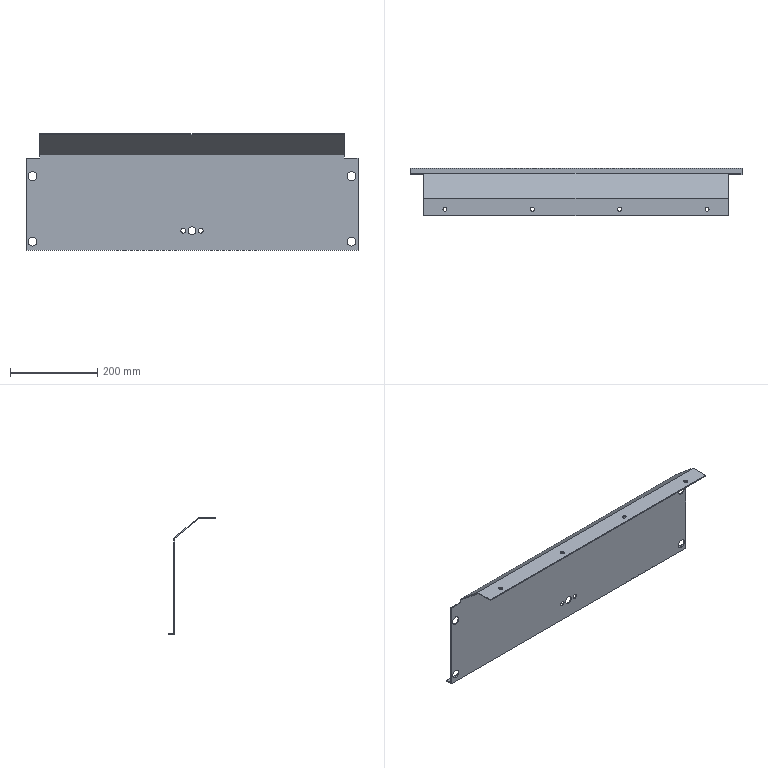Part | SolidWorks | features BaseBody 1 | 1 solid | 38 faces | box 760 x 109.5 x 267.5 mm | volume 630879 mm3 | cylinder 22 | plane 16 | commonest cylinder face diameters 9.1 x8 20 x8 11 x4 18 x2
STEP:
#1=CARTESIAN_POINT('',(181.946,-3035.973,2024.971));
#2=VERTEX_POINT('',#1);
#3=CARTESIAN_POINT('',(181.946,-3035.973,2004.971));
#4=VERTEX_POINT('',#3);
#5=CARTESIAN_POINT('',(181.946,-3035.973,2014.971));
#6=DIRECTION('',(0.,-1.,0.));
#7=DIRECTION('',(0.,0.,-1.));
#8=AXIS2_PLACEMENT_3D('',#5,#6,#7);
#9=CIRCLE('',#8,10.);
#10=EDGE_CURVE('',#2,#4,#9,.T.);
#11=ORIENTED_EDGE('',*,*,#10,.F.);
#12=CARTESIAN_POINT('',(181.946,-3038.473,2024.971));
#13=VERTEX_POINT('',#12);
#14=CARTESIAN_POINT('',(181.946,-3041.02,2024.971));
#15=DIRECTION('',(0.,-1.,0.));
#16=VECTOR('',#15,1000.);
#17=LINE('',#14,#16);
#18=EDGE_CURVE('',#2,#13,#17,.T.);
#19=ORIENTED_EDGE('',*,*,#18,.T.);
#20=CARTESIAN_POINT('',(181.946,-3038.473,2004.971));
#21=VERTEX_POINT('',#20);
#22=CARTESIAN_POINT('',(181.946,-3038.473,2014.971));
#23=DIRECTION('',(0.,1.,0.));
#24=DIRECTION('',(0.,0.,-1.));
#25=AXIS2_PLACEMENT_3D('',#22,#23,#24);
#26=CIRCLE('',#25,10.);
#27=EDGE_CURVE('',#21,#13,#26,.T.);
#28=ORIENTED_EDGE('',*,*,#27,.F.);
#29=CARTESIAN_POINT('',(181.946,-3041.02,2004.971));
#30=DIRECTION('',(0.,-1.,0.));
#31=VECTOR('',#30,1000.);
#32=LINE('',#29,#31);
#33=EDGE_CURVE('',#4,#21,#32,.T.);
#34=ORIENTED_EDGE('',*,*,#33,.F.);
#35=EDGE_LOOP('',(#11,#19,#28,#34));
#36=FACE_OUTER_BOUND('',#35,.T.);
#37=CARTESIAN_POINT('',(181.946,-3041.02,2014.971));
#38=DIRECTION('',(0.,-1.,0.));
#39=DIRECTION('',(0.,0.,-1.));
#40=AXIS2_PLACEMENT_3D('',#37,#38,#39);
#41=CYLINDRICAL_SURFACE('',#40,10.);
#42=ADVANCED_FACE('',(#36),#41,.F.);
#43=CARTESIAN_POINT('',(911.946,-3038.473,2004.971));
#44=VERTEX_POINT('',#43);
#45=CARTESIAN_POINT('',(911.946,-3038.473,2024.971));
#46=VERTEX_POINT('',#45);
#47=CARTESIAN_POINT('',(911.946,-3038.473,2014.971));
#48=DIRECTION('',(0.,1.,0.));
#49=DIRECTION('',(0.,0.,1.));
#50=AXIS2_PLACEMENT_3D('',#47,#48,#49);
#51=CIRCLE('',#50,10.);
#52=EDGE_CURVE('',#44,#46,#51,.T.);
#53=ORIENTED_EDGE('',*,*,#52,.F.);
#54=CARTESIAN_POINT('',(911.946,-3035.973,2004.971));
#55=VERTEX_POINT('',#54);
#56=CARTESIAN_POINT('',(911.946,-3041.02,2004.971));
#57=DIRECTION('',(0.,1.,0.));
#58=VECTOR('',#57,1000.);
#59=LINE('',#56,#58);
#60=EDGE_CURVE('',#44,#55,#59,.T.);
#61=ORIENTED_EDGE('',*,*,#60,.T.);
#62=CARTESIAN_POINT('',(911.946,-3035.973,2024.971));
#63=VERTEX_POINT('',#62);
#64=CARTESIAN_POINT('',(911.946,-3035.973,2014.971));
#65=DIRECTION('',(0.,-1.,0.));
#66=DIRECTION('',(0.,0.,1.));
#67=AXIS2_PLACEMENT_3D('',#64,#65,#66);
#68=CIRCLE('',#67,10.);
#69=EDGE_CURVE('',#63,#55,#68,.T.);
#70=ORIENTED_EDGE('',*,*,#69,.F.);
#71=CARTESIAN_POINT('',(911.946,-3041.02,2024.971));
#72=DIRECTION('',(0.,1.,0.));
#73=VECTOR('',#72,1000.);
#74=LINE('',#71,#73);
#75=EDGE_CURVE('',#46,#63,#74,.T.);
#76=ORIENTED_EDGE('',*,*,#75,.F.);
#77=EDGE_LOOP('',(#53,#61,#70,#76));
#78=FACE_OUTER_BOUND('',#77,.T.);
#79=CARTESIAN_POINT('',(911.946,-3041.02,2014.971));
#80=DIRECTION('',(0.,1.,0.));
#81=DIRECTION('',(0.,0.,1.));
#82=AXIS2_PLACEMENT_3D('',#79,#80,#81);
#83=CYLINDRICAL_SURFACE('',#82,10.);
#84=ADVANCED_FACE('',(#78),#83,.F.);
#85=CARTESIAN_POINT('',(911.946,-3038.473,1854.971));
#86=VERTEX_POINT('',#85);
#87=CARTESIAN_POINT('',(911.946,-3038.473,1874.971));
#88=VERTEX_POINT('',#87);
#89=CARTESIAN_POINT('',(911.946,-3038.473,1864.971));
#90=DIRECTION('',(0.,1.,0.));
#91=DIRECTION('',(0.,0.,1.));
#92=AXIS2_PLACEMENT_3D('',#89,#90,#91);
#93=CIRCLE('',#92,10.);
#94=EDGE_CURVE('',#86,#88,#93,.T.);
#95=ORIENTED_EDGE('',*,*,#94,.F.);
#96=CARTESIAN_POINT('',(911.946,-3035.973,1854.971));
#97=VERTEX_POINT('',#96);
#98=CARTESIAN_POINT('',(911.946,-3041.02,1854.971));
#99=DIRECTION('',(0.,1.,0.));
#100=VECTOR('',#99,1000.);
#101=LINE('',#98,#100);
#102=EDGE_CURVE('',#86,#97,#101,.T.);
#103=ORIENTED_EDGE('',*,*,#102,.T.);
#104=CARTESIAN_POINT('',(911.946,-3035.973,1874.971));
#105=VERTEX_POINT('',#104);
#106=CARTESIAN_POINT('',(911.946,-3035.973,1864.971));
#107=DIRECTION('',(0.,-1.,0.));
#108=DIRECTION('',(0.,0.,1.));
#109=AXIS2_PLACEMENT_3D('',#106,#107,#108);
#110=CIRCLE('',#109,10.);
#111=EDGE_CURVE('',#105,#97,#110,.T.);
#112=ORIENTED_EDGE('',*,*,#111,.F.);
#113=CARTESIAN_POINT('',(911.946,-3041.02,1874.971));
#114=DIRECTION('',(0.,1.,0.));
#115=VECTOR('',#114,1000.);
#116=LINE('',#113,#115);
#117=EDGE_CURVE('',#88,#105,#116,.T.);
#118=ORIENTED_EDGE('',*,*,#117,.F.);
#119=EDGE_LOOP('',(#95,#103,#112,#118));
#120=FACE_OUTER_BOUND('',#119,.T.);
#121=CARTESIAN_POINT('',(911.946,-3041.02,1864.971));
#122=DIRECTION('',(0.,1.,0.));
#123=DIRECTION('',(0.,0.,1.));
#124=AXIS2_PLACEMENT_3D('',#121,#122,#123);
#125=CYLINDRICAL_SURFACE('',#124,10.);
#126=ADVANCED_FACE('',(#120),#125,.F.);
#127=CARTESIAN_POINT('',(181.946,-3035.973,1874.971));
#128=VERTEX_POINT('',#127);
#129=CARTESIAN_POINT('',(181.946,-3035.973,1854.971));
#130=VERTEX_POINT('',#129);
#131=CARTESIAN_POINT('',(181.946,-3035.973,1864.971));
#132=DIRECTION('',(0.,-1.,0.));
#133=DIRECTION('',(0.,0.,-1.));
#134=AXIS2_PLACEMENT_3D('',#131,#132,#133);
#135=CIRCLE('',#134,10.);
#136=EDGE_CURVE('',#128,#130,#135,.T.);
#137=ORIENTED_EDGE('',*,*,#136,.F.);
#138=CARTESIAN_POINT('',(181.946,-3038.473,1874.971));
#139=VERTEX_POINT('',#138);
#140=CARTESIAN_POINT('',(181.946,-3041.02,1874.971));
#141=DIRECTION('',(0.,-1.,0.));
#142=VECTOR('',#141,1000.);
#143=LINE('',#140,#142);
#144=EDGE_CURVE('',#128,#139,#143,.T.);
#145=ORIENTED_EDGE('',*,*,#144,.T.);
#146=CARTESIAN_POINT('',(181.946,-3038.473,1854.971));
#147=VERTEX_POINT('',#146);
#148=CARTESIAN_POINT('',(181.946,-3038.473,1864.971));
#149=DIRECTION('',(0.,1.,0.));
#150=DIRECTION('',(0.,0.,-1.));
#151=AXIS2_PLACEMENT_3D('',#148,#149,#150);
#152=CIRCLE('',#151,10.);
#153=EDGE_CURVE('',#147,#139,#152,.T.);
#154=ORIENTED_EDGE('',*,*,#153,.F.);
#155=CARTESIAN_POINT('',(181.946,-3041.02,1854.971));
#156=DIRECTION('',(0.,-1.,0.));
#157=VECTOR('',#156,1000.);
#158=LINE('',#155,#157);
#159=EDGE_CURVE('',#130,#147,#158,.T.);
#160=ORIENTED_EDGE('',*,*,#159,.F.);
#161=EDGE_LOOP('',(#137,#145,#154,#160));
#162=FACE_OUTER_BOUND('',#161,.T.);
#163=CARTESIAN_POINT('',(181.946,-3041.02,1864.971));
#164=DIRECTION('',(0.,-1.,0.));
#165=DIRECTION('',(0.,0.,-1.));
#166=AXIS2_PLACEMENT_3D('',#163,#164,#165);
#167=CYLINDRICAL_SURFACE('',#166,10.);
#168=ADVANCED_FACE('',(#162),#167,.F.);
#169=CARTESIAN_POINT('',(526.946,-3035.973,1895.471));
#170=VERTEX_POINT('',#169);
#171=CARTESIAN_POINT('',(526.946,-3035.973,1884.471));
#172=VERTEX_POINT('',#171);
#173=CARTESIAN_POINT('',(526.946,-3035.973,1889.971));
#174=DIRECTION('',(0.,-1.,0.));
#175=DIRECTION('',(0.,0.,-1.));
#176=AXIS2_PLACEMENT_3D('',#173,#174,#175);
#177=CIRCLE('',#176,5.5);
#178=EDGE_CURVE('',#170,#172,#177,.T.);
#179=ORIENTED_EDGE('',*,*,#178,.F.);
#180=CARTESIAN_POINT('',(526.946,-3038.473,1895.471));
#181=VERTEX_POINT('',#180);
#182=CARTESIAN_POINT('',(526.946,-3062.639,1895.471));
#183=DIRECTION('',(0.,-1.,0.));
#184=VECTOR('',#183,1000.);
#185=LINE('',#182,#184);
#186=EDGE_CURVE('',#170,#181,#185,.T.);
#187=ORIENTED_EDGE('',*,*,#186,.T.);
#188=CARTESIAN_POINT('',(526.946,-3038.473,1884.471));
#189=VERTEX_POINT('',#188);
#190=CARTESIAN_POINT('',(526.946,-3038.473,1889.971));
#191=DIRECTION('',(0.,1.,0.));
#192=DIRECTION('',(0.,0.,-1.));
#193=AXIS2_PLACEMENT_3D('',#190,#191,#192);
#194=CIRCLE('',#193,5.5);
#195=EDGE_CURVE('',#189,#181,#194,.T.);
#196=ORIENTED_EDGE('',*,*,#195,.F.);
#197=CARTESIAN_POINT('',(526.946,-3062.639,1884.471));
#198=DIRECTION('',(0.,-1.,0.));
#199=VECTOR('',#198,1000.);
#200=LINE('',#197,#199);
#201=EDGE_CURVE('',#172,#189,#200,.T.);
#202=ORIENTED_EDGE('',*,*,#201,.F.);
#203=EDGE_LOOP('',(#179,#187,#196,#202));
#204=FACE_OUTER_BOUND('',#203,.T.);
#205=CARTESIAN_POINT('',(526.946,-3062.639,1889.971));
#206=DIRECTION('',(0.,-1.,0.));
#207=DIRECTION('',(0.,0.,-1.));
#208=AXIS2_PLACEMENT_3D('',#205,#206,#207);
#209=CYLINDRICAL_SURFACE('',#208,5.5);
#210=ADVANCED_FACE('',(#204),#209,.F.);
#211=CARTESIAN_POINT('',(566.946,-3038.473,1884.471));
#212=VERTEX_POINT('',#211);
#213=CARTESIAN_POINT('',(566.946,-3038.473,1895.471));
#214=VERTEX_POINT('',#213);
#215=CARTESIAN_POINT('',(566.946,-3038.473,1889.971));
#216=DIRECTION('',(0.,1.,0.));
#217=DIRECTION('',(0.,0.,1.));
#218=AXIS2_PLACEMENT_3D('',#215,#216,#217);
#219=CIRCLE('',#218,5.5);
#220=EDGE_CURVE('',#212,#214,#219,.T.);
#221=ORIENTED_EDGE('',*,*,#220,.F.);
#222=CARTESIAN_POINT('',(566.946,-3035.973,1884.471));
#223=VERTEX_POINT('',#222);
#224=CARTESIAN_POINT('',(566.946,-3062.639,1884.471));
#225=DIRECTION('',(0.,1.,0.));
#226=VECTOR('',#225,1000.);
#227=LINE('',#224,#226);
#228=EDGE_CURVE('',#212,#223,#227,.T.);
#229=ORIENTED_EDGE('',*,*,#228,.T.);
#230=CARTESIAN_POINT('',(566.946,-3035.973,1895.471));
#231=VERTEX_POINT('',#230);
#232=CARTESIAN_POINT('',(566.946,-3035.973,1889.971));
#233=DIRECTION('',(0.,-1.,0.));
#234=DIRECTION('',(0.,0.,1.));
#235=AXIS2_PLACEMENT_3D('',#232,#233,#234);
#236=CIRCLE('',#235,5.5);
#237=EDGE_CURVE('',#231,#223,#236,.T.);
#238=ORIENTED_EDGE('',*,*,#237,.F.);
#239=CARTESIAN_POINT('',(566.946,-3062.639,1895.471));
#240=DIRECTION('',(0.,1.,0.));
#241=VECTOR('',#240,1000.);
#242=LINE('',#239,#241);
#243=EDGE_CURVE('',#214,#231,#242,.T.);
#244=ORIENTED_EDGE('',*,*,#243,.F.);
#245=EDGE_LOOP('',(#221,#229,#238,#244));
#246=FACE_OUTER_BOUND('',#245,.T.);
#247=CARTESIAN_POINT('',(566.946,-3062.639,1889.971));
#248=DIRECTION('',(0.,1.,0.));
#249=DIRECTION('',(0.,0.,1.));
#250=AXIS2_PLACEMENT_3D('',#247,#248,#249);
#251=CYLINDRICAL_SURFACE('',#250,5.5);
#252=ADVANCED_FACE('',(#246),#251,.F.);
#253=CARTESIAN_POINT('',(546.946,-3035.973,1898.971));
#254=VERTEX_POINT('',#253);
#255=CARTESIAN_POINT('',(546.946,-3035.973,1880.971));
#256=VERTEX_POINT('',#255);
#257=CARTESIAN_POINT('',(546.946,-3035.973,1889.971));
#258=DIRECTION('',(0.,-1.,0.));
#259=DIRECTION('',(0.,0.,-1.));
#260=AXIS2_PLACEMENT_3D('',#257,#258,#259);
#261=CIRCLE('',#260,9.);
#262=EDGE_CURVE('',#254,#256,#261,.T.);
#263=ORIENTED_EDGE('',*,*,#262,.F.);
#264=CARTESIAN_POINT('',(546.946,-3038.473,1898.971));
#265=VERTEX_POINT('',#264);
#266=CARTESIAN_POINT('',(546.946,-3051.149,1898.971));
#267=DIRECTION('',(0.,-1.,0.));
#268=VECTOR('',#267,1000.);
#269=LINE('',#266,#268);
#270=EDGE_CURVE('',#254,#265,#269,.T.);
#271=ORIENTED_EDGE('',*,*,#270,.T.);
#272=CARTESIAN_POINT('',(546.946,-3038.473,1880.971));
#273=VERTEX_POINT('',#272);
#274=CARTESIAN_POINT('',(546.946,-3038.473,1889.971));
#275=DIRECTION('',(0.,1.,0.));
#276=DIRECTION('',(0.,0.,-1.));
#277=AXIS2_PLACEMENT_3D('',#274,#275,#276);
#278=CIRCLE('',#277,9.);
#279=EDGE_CURVE('',#273,#265,#278,.T.);
#280=ORIENTED_EDGE('',*,*,#279,.F.);
#281=CARTESIAN_POINT('',(546.946,-3051.149,1880.971));
#282=DIRECTION('',(0.,-1.,0.));
#283=VECTOR('',#282,1000.);
#284=LINE('',#281,#283);
#285=EDGE_CURVE('',#256,#273,#284,.T.);
#286=ORIENTED_EDGE('',*,*,#285,.F.);
#287=EDGE_LOOP('',(#263,#271,#280,#286));
#288=FACE_OUTER_BOUND('',#287,.T.);
#289=CARTESIAN_POINT('',(546.946,-3051.149,1889.971));
#290=DIRECTION('',(0.,-1.,0.));
#291=DIRECTION('',(0.,0.,-1.));
#292=AXIS2_PLACEMENT_3D('',#289,#290,#291);
#293=CYLINDRICAL_SURFACE('',#292,9.);
#294=ADVANCED_FACE('',(#288),#293,.F.);
#295=CARTESIAN_POINT('',(442.396,-3117.973,2109.971));
#296=VERTEX_POINT('',#295);
#297=CARTESIAN_POINT('',(451.496,-3117.973,2109.971));
#298=VERTEX_POINT('',#297);
#299=CARTESIAN_POINT('',(446.946,-3117.973,2109.971));
#300=DIRECTION('',(0.,0.,1.));
#301=DIRECTION('',(1.,0.,0.));
#302=AXIS2_PLACEMENT_3D('',#299,#300,#301);
#303=CIRCLE('',#302,4.55);
#304=EDGE_CURVE('',#296,#298,#303,.T.);
#305=ORIENTED_EDGE('',*,*,#304,.F.);
#306=CARTESIAN_POINT('',(442.396,-3117.973,2112.471));
#307=VERTEX_POINT('',#306);
#308=CARTESIAN_POINT('',(442.396,-3117.973,2106.225));
#309=DIRECTION('',(0.,0.,1.));
#310=VECTOR('',#309,1000.);
#311=LINE('',#308,#310);
#312=EDGE_CURVE('',#296,#307,#311,.T.);
#313=ORIENTED_EDGE('',*,*,#312,.T.);
#314=CARTESIAN_POINT('',(451.496,-3117.973,2112.471));
#315=VERTEX_POINT('',#314);
#316=CARTESIAN_POINT('',(446.946,-3117.973,2112.471));
#317=DIRECTION('',(0.,0.,-1.));
#318=DIRECTION('',(1.,0.,0.));
#319=AXIS2_PLACEMENT_3D('',#316,#317,#318);
#320=CIRCLE('',#319,4.55);
#321=EDGE_CURVE('',#315,#307,#320,.T.);
#322=ORIENTED_EDGE('',*,*,#321,.F.);
#323=CARTESIAN_POINT('',(451.496,-3117.973,2106.225));
#324=DIRECTION('',(0.,0.,1.));
#325=VECTOR('',#324,1000.);
#326=LINE('',#323,#325);
#327=EDGE_CURVE('',#298,#315,#326,.T.);
#328=ORIENTED_EDGE('',*,*,#327,.F.);
#329=EDGE_LOOP('',(#305,#313,#322,#328));
#330=FACE_OUTER_BOUND('',#329,.T.);
#331=CARTESIAN_POINT('',(446.946,-3117.973,2106.225));
#332=DIRECTION('',(0.,0.,1.));
#333=DIRECTION('',(1.,0.,0.));
#334=AXIS2_PLACEMENT_3D('',#331,#332,#333);
#335=CYLINDRICAL_SURFACE('',#334,4.55);
#336=ADVANCED_FACE('',(#330),#335,.F.);
#337=CARTESIAN_POINT('',(651.496,-3117.973,2112.471));
#338=VERTEX_POINT('',#337);
#339=CARTESIAN_POINT('',(642.396,-3117.973,2112.471));
#340=VERTEX_POINT('',#339);
#341=CARTESIAN_POINT('',(646.946,-3117.973,2112.471));
#342=DIRECTION('',(0.,0.,-1.));
#343=DIRECTION('',(-1.,0.,0.));
#344=AXIS2_PLACEMENT_3D('',#341,#342,#343);
#345=CIRCLE('',#344,4.55);
#346=EDGE_CURVE('',#338,#340,#345,.T.);
#347=ORIENTED_EDGE('',*,*,#346,.F.);
#348=CARTESIAN_POINT('',(651.496,-3117.973,2109.971));
#349=VERTEX_POINT('',#348);
#350=CARTESIAN_POINT('',(651.496,-3117.973,2106.225));
#351=DIRECTION('',(0.,0.,-1.));
#352=VECTOR('',#351,1000.);
#353=LINE('',#350,#352);
#354=EDGE_CURVE('',#338,#349,#353,.T.);
#355=ORIENTED_EDGE('',*,*,#354,.T.);
#356=CARTESIAN_POINT('',(642.396,-3117.973,2109.971));
#357=VERTEX_POINT('',#356);
#358=CARTESIAN_POINT('',(646.946,-3117.973,2109.971));
#359=DIRECTION('',(0.,0.,1.));
#360=DIRECTION('',(-1.,0.,0.));
#361=AXIS2_PLACEMENT_3D('',#358,#359,#360);
#362=CIRCLE('',#361,4.55);
#363=EDGE_CURVE('',#357,#349,#362,.T.);
#364=ORIENTED_EDGE('',*,*,#363,.F.);
#365=CARTESIAN_POINT('',(642.396,-3117.973,2106.225));
#366=DIRECTION('',(0.,0.,-1.));
#367=VECTOR('',#366,1000.);
#368=LINE('',#365,#367);
#369=EDGE_CURVE('',#340,#357,#368,.T.);
#370=ORIENTED_EDGE('',*,*,#369,.F.);
#371=EDGE_LOOP('',(#347,#355,#364,#370));
#372=FACE_OUTER_BOUND('',#371,.T.);
#373=CARTESIAN_POINT('',(646.946,-3117.973,2106.225));
#374=DIRECTION('',(0.,0.,-1.));
#375=DIRECTION('',(-1.,0.,0.));
#376=AXIS2_PLACEMENT_3D('',#373,#374,#375);
#377=CYLINDRICAL_SURFACE('',#376,4.55);
#378=ADVANCED_FACE('',(#372),#377,.F.);
#379=CARTESIAN_POINT('',(851.496,-3117.973,2112.471));
#380=VERTEX_POINT('',#379);
#381=CARTESIAN_POINT('',(842.396,-3117.973,2112.471));
#382=VERTEX_POINT('',#381);
#383=CARTESIAN_POINT('',(846.946,-3117.973,2112.471));
#384=DIRECTION('',(0.,0.,-1.));
#385=DIRECTION('',(-1.,0.,0.));
#386=AXIS2_PLACEMENT_3D('',#383,#384,#385);
#387=CIRCLE('',#386,4.55);
#388=EDGE_CURVE('',#380,#382,#387,.T.);
#389=ORIENTED_EDGE('',*,*,#388,.F.);
#390=CARTESIAN_POINT('',(851.496,-3117.973,2109.971));
#391=VERTEX_POINT('',#390);
#392=CARTESIAN_POINT('',(851.496,-3117.973,2106.225));
#393=DIRECTION('',(0.,0.,-1.));
#394=VECTOR('',#393,1000.);
#395=LINE('',#392,#394);
#396=EDGE_CURVE('',#380,#391,#395,.T.);
#397=ORIENTED_EDGE('',*,*,#396,.T.);
#398=CARTESIAN_POINT('',(842.396,-3117.973,2109.971));
#399=VERTEX_POINT('',#398);
#400=CARTESIAN_POINT('',(846.946,-3117.973,2109.971));
#401=DIRECTION('',(0.,0.,1.));
#402=DIRECTION('',(-1.,0.,0.));
#403=AXIS2_PLACEMENT_3D('',#400,#401,#402);
#404=CIRCLE('',#403,4.55);
#405=EDGE_CURVE('',#399,#391,#404,.T.);
#406=ORIENTED_EDGE('',*,*,#405,.F.);
#407=CARTESIAN_POINT('',(842.396,-3117.973,2106.225));
#408=DIRECTION('',(0.,0.,-1.));
#409=VECTOR('',#408,1000.);
#410=LINE('',#407,#409);
#411=EDGE_CURVE('',#382,#399,#410,.T.);
#412=ORIENTED_EDGE('',*,*,#411,.F.);
#413=EDGE_LOOP('',(#389,#397,#406,#412));
#414=FACE_OUTER_BOUND('',#413,.T.);
#415=CARTESIAN_POINT('',(846.946,-3117.973,2106.225));
#416=DIRECTION('',(0.,0.,-1.));
#417=DIRECTION('',(-1.,0.,0.));
#418=AXIS2_PLACEMENT_3D('',#415,#416,#417);
#419=CYLINDRICAL_SURFACE('',#418,4.55);
#420=ADVANCED_FACE('',(#414),#419,.F.);
#421=CARTESIAN_POINT('',(242.396,-3117.973,2109.971));
#422=VERTEX_POINT('',#421);
#423=CARTESIAN_POINT('',(251.496,-3117.973,2109.971));
#424=VERTEX_POINT('',#423);
#425=CARTESIAN_POINT('',(246.946,-3117.973,2109.971));
#426=DIRECTION('',(0.,0.,1.));
#427=DIRECTION('',(1.,0.,0.));
#428=AXIS2_PLACEMENT_3D('',#425,#426,#427);
#429=CIRCLE('',#428,4.55);
#430=EDGE_CURVE('',#422,#424,#429,.T.);
#431=ORIENTED_EDGE('',*,*,#430,.F.);
#432=CARTESIAN_POINT('',(242.396,-3117.973,2112.471));
#433=VERTEX_POINT('',#432);
#434=CARTESIAN_POINT('',(242.396,-3117.973,2106.225));
#435=DIRECTION('',(0.,0.,1.));
#436=VECTOR('',#435,1000.);
#437=LINE('',#434,#436);
#438=EDGE_CURVE('',#422,#433,#437,.T.);
#439=ORIENTED_EDGE('',*,*,#438,.T.);
#440=CARTESIAN_POINT('',(251.496,-3117.973,2112.471));
#441=VERTEX_POINT('',#440);
#442=CARTESIAN_POINT('',(246.946,-3117.973,2112.471));
#443=DIRECTION('',(0.,0.,-1.));
#444=DIRECTION('',(1.,0.,0.));
#445=AXIS2_PLACEMENT_3D('',#442,#443,#444);
#446=CIRCLE('',#445,4.55);
#447=EDGE_CURVE('',#441,#433,#446,.T.);
#448=ORIENTED_EDGE('',*,*,#447,.F.);
#449=CARTESIAN_POINT('',(251.496,-3117.973,2106.225));
#450=DIRECTION('',(0.,0.,1.));
#451=VECTOR('',#450,1000.);
#452=LINE('',#449,#451);
#453=EDGE_CURVE('',#424,#441,#452,.T.);
#454=ORIENTED_EDGE('',*,*,#453,.F.);
#455=EDGE_LOOP('',(#431,#439,#448,#454));
#456=FACE_OUTER_BOUND('',#455,.T.);
#457=CARTESIAN_POINT('',(246.946,-3117.973,2106.225));
#458=DIRECTION('',(0.,0.,1.));
#459=DIRECTION('',(1.,0.,0.));
#460=AXIS2_PLACEMENT_3D('',#457,#458,#459);
#461=CYLINDRICAL_SURFACE('',#460,4.55);
#462=ADVANCED_FACE('',(#456),#461,.F.);
#463=CARTESIAN_POINT('',(895.446,-3038.473,2056.471));
#464=VERTEX_POINT('',#463);
#465=CARTESIAN_POINT('',(895.446,-3038.473,2063.8));
#466=VERTEX_POINT('',#465);
#467=CARTESIAN_POINT('',(895.446,-3038.473,1847.471));
#468=DIRECTION('',(0.,0.,1.));
#469=VECTOR('',#468,1000.);
#470=LINE('',#467,#469);
#471=EDGE_CURVE('',#464,#466,#470,.T.);
#472=ORIENTED_EDGE('',*,*,#471,.T.);
#473=CARTESIAN_POINT('',(198.446,-3038.473,2063.8));
#474=VERTEX_POINT('',#473);
#475=CARTESIAN_POINT('',(926.946,-3038.473,2063.8));
#476=DIRECTION('',(-1.,0.,0.));
#477=VECTOR('',#476,1000.);
#478=LINE('',#475,#477);
#479=EDGE_CURVE('',#466,#474,#478,.T.);
#480=ORIENTED_EDGE('',*,*,#479,.T.);
#481=CARTESIAN_POINT('',(198.446,-3038.473,2056.471));
#482=VERTEX_POINT('',#481);
#483=CARTESIAN_POINT('',(198.446,-3038.473,1847.471));
#484=DIRECTION('',(0.,0.,-1.));
#485=VECTOR('',#484,1000.);
#486=LINE('',#483,#485);
#487=EDGE_CURVE('',#474,#482,#486,.T.);
#488=ORIENTED_EDGE('',*,*,#487,.T.);
#489=CARTESIAN_POINT('',(166.946,-3038.473,2056.471));
#490=VERTEX_POINT('',#489);
#491=CARTESIAN_POINT('',(926.946,-3038.473,2056.471));
#492=DIRECTION('',(-1.,0.,0.));
#493=VECTOR('',#492,1000.);
#494=LINE('',#491,#493);
#495=EDGE_CURVE('',#482,#490,#494,.T.);
#496=ORIENTED_EDGE('',*,*,#495,.T.);
#497=CARTESIAN_POINT('',(166.946,-3038.473,1844.971));
#498=VERTEX_POINT('',#497);
#499=CARTESIAN_POINT('',(166.946,-3038.473,1847.471));
#500=DIRECTION('',(0.,0.,-1.));
#501=VECTOR('',#500,1000.);
#502=LINE('',#499,#501);
#503=EDGE_CURVE('',#490,#498,#502,.T.);
#504=ORIENTED_EDGE('',*,*,#503,.T.);
#505=CARTESIAN_POINT('',(926.946,-3038.473,1844.971));
#506=VERTEX_POINT('',#505);
#507=CARTESIAN_POINT('',(926.946,-3038.473,1844.971));
#508=DIRECTION('',(1.,0.,0.));
#509=VECTOR('',#508,1000.);
#510=LINE('',#507,#509);
#511=EDGE_CURVE('',#498,#506,#510,.T.);
#512=ORIENTED_EDGE('',*,*,#511,.T.);
#513=CARTESIAN_POINT('',(926.946,-3038.473,2056.471));
#514=VERTEX_POINT('',#513);
#515=CARTESIAN_POINT('',(926.946,-3038.473,1847.471));
#516=DIRECTION('',(0.,0.,1.));
#517=VECTOR('',#516,1000.);
#518=LINE('',#515,#517);
#519=EDGE_CURVE('',#506,#514,#518,.T.);
#520=ORIENTED_EDGE('',*,*,#519,.T.);
#521=CARTESIAN_POINT('',(926.946,-3038.473,2056.471));
#522=DIRECTION('',(-1.,0.,0.));
#523=VECTOR('',#522,1000.);
#524=LINE('',#521,#523);
#525=EDGE_CURVE('',#514,#464,#524,.T.);
#526=ORIENTED_EDGE('',*,*,#525,.T.);
#527=EDGE_LOOP('',(#472,#480,#488,#496,#504,#512,#520,#526));
#528=FACE_OUTER_BOUND('',#527,.T.);
#529=ORIENTED_EDGE('',*,*,#27,.T.);
#530=CARTESIAN_POINT('',(181.946,-3038.473,2014.971));
#531=DIRECTION('',(0.,1.,0.));
#532=DIRECTION('',(0.,0.,-1.));
#533=AXIS2_PLACEMENT_3D('',#530,#531,#532);
#534=CIRCLE('',#533,10.);
#535=EDGE_CURVE('',#13,#21,#534,.T.);
#536=ORIENTED_EDGE('',*,*,#535,.T.);
#537=EDGE_LOOP('',(#529,#536));
#538=FACE_BOUND('',#537,.T.);
#539=CARTESIAN_POINT('',(911.946,-3038.473,2014.971));
#540=DIRECTION('',(0.,1.,0.));
#541=DIRECTION('',(0.,0.,1.));
#542=AXIS2_PLACEMENT_3D('',#539,#540,#541);
#543=CIRCLE('',#542,10.);
#544=EDGE_CURVE('',#46,#44,#543,.T.);
#545=ORIENTED_EDGE('',*,*,#544,.T.);
#546=ORIENTED_EDGE('',*,*,#52,.T.);
#547=EDGE_LOOP('',(#545,#546));
#548=FACE_BOUND('',#547,.T.);
#549=CARTESIAN_POINT('',(911.946,-3038.473,1864.971));
#550=DIRECTION('',(0.,1.,0.));
#551=DIRECTION('',(0.,0.,1.));
#552=AXIS2_PLACEMENT_3D('',#549,#550,#551);
#553=CIRCLE('',#552,10.);
#554=EDGE_CURVE('',#88,#86,#553,.T.);
#555=ORIENTED_EDGE('',*,*,#554,.T.);
#556=ORIENTED_EDGE('',*,*,#94,.T.);
#557=EDGE_LOOP('',(#555,#556));
#558=FACE_BOUND('',#557,.T.);
#559=ORIENTED_EDGE('',*,*,#153,.T.);
#560=CARTESIAN_POINT('',(181.946,-3038.473,1864.971));
#561=DIRECTION('',(0.,1.,0.));
#562=DIRECTION('',(0.,0.,-1.));
#563=AXIS2_PLACEMENT_3D('',#560,#561,#562);
#564=CIRCLE('',#563,10.);
#565=EDGE_CURVE('',#139,#147,#564,.T.);
#566=ORIENTED_EDGE('',*,*,#565,.T.);
#567=EDGE_LOOP('',(#559,#566));
#568=FACE_BOUND('',#567,.T.);
#569=ORIENTED_EDGE('',*,*,#195,.T.);
#570=CARTESIAN_POINT('',(526.946,-3038.473,1889.971));
#571=DIRECTION('',(0.,1.,0.));
#572=DIRECTION('',(0.,0.,-1.));
#573=AXIS2_PLACEMENT_3D('',#570,#571,#572);
#574=CIRCLE('',#573,5.5);
#575=EDGE_CURVE('',#181,#189,#574,.T.);
#576=ORIENTED_EDGE('',*,*,#575,.T.);
#577=EDGE_LOOP('',(#569,#576));
#578=FACE_BOUND('',#577,.T.);
#579=CARTESIAN_POINT('',(566.946,-3038.473,1889.971));
#580=DIRECTION('',(0.,1.,0.));
#581=DIRECTION('',(0.,0.,1.));
#582=AXIS2_PLACEMENT_3D('',#579,#580,#581);
#583=CIRCLE('',#582,5.5);
#584=EDGE_CURVE('',#214,#212,#583,.T.);
#585=ORIENTED_EDGE('',*,*,#584,.T.);
#586=ORIENTED_EDGE('',*,*,#220,.T.);
#587=EDGE_LOOP('',(#585,#586));
#588=FACE_BOUND('',#587,.T.);
#589=ORIENTED_EDGE('',*,*,#279,.T.);
#590=CARTESIAN_POINT('',(546.946,-3038.473,1889.971));
#591=DIRECTION('',(0.,1.,0.));
#592=DIRECTION('',(0.,0.,-1.));
#593=AXIS2_PLACEMENT_3D('',#590,#591,#592);
#594=CIRCLE('',#593,9.);
#595=EDGE_CURVE('',#265,#273,#594,.T.);
#596=ORIENTED_EDGE('',*,*,#595,.T.);
#597=EDGE_LOOP('',(#589,#596));
#598=FACE_BOUND('',#597,.T.);
#599=CARTESIAN_POINT('',(926.946,-3038.473,1847.471));
#600=DIRECTION('',(0.,-1.,0.));
#601=DIRECTION('',(0.,0.,-1.));
#602=AXIS2_PLACEMENT_3D('',#599,#600,#601);
#603=PLANE('',#602);
#604=ADVANCED_FACE('',(#528,#538,#548,#558,#568,#578,#588,#598),#603,.T.);
#605=CARTESIAN_POINT('',(895.446,-3093.878,2109.971));
#606=VERTEX_POINT('',#605);
#607=CARTESIAN_POINT('',(895.446,-3093.878,2109.971));
#608=DIRECTION('',(0.,-0.7682,0.6402));
#609=VECTOR('',#608,1000.);
#610=LINE('',#607,#609);
#611=EDGE_CURVE('',#466,#606,#610,.T.);
#612=ORIENTED_EDGE('',*,*,#611,.T.);
#613=CARTESIAN_POINT('',(198.446,-3093.878,2109.971));
#614=VERTEX_POINT('',#613);
#615=CARTESIAN_POINT('',(926.946,-3093.878,2109.971));
#616=DIRECTION('',(-1.,0.,0.));
#617=VECTOR('',#616,1000.);
#618=LINE('',#615,#617);
#619=EDGE_CURVE('',#606,#614,#618,.T.);
#620=ORIENTED_EDGE('',*,*,#619,.T.);
#621=CARTESIAN_POINT('',(198.446,-3093.878,2109.971));
#622=DIRECTION('',(0.,0.7682,-0.6402));
#623=VECTOR('',#622,1000.);
#624=LINE('',#621,#623);
#625=EDGE_CURVE('',#614,#474,#624,.T.);
#626=ORIENTED_EDGE('',*,*,#625,.T.);
#627=ORIENTED_EDGE('',*,*,#479,.F.);
#628=EDGE_LOOP('',(#612,#620,#626,#627));
#629=FACE_OUTER_BOUND('',#628,.T.);
#630=CARTESIAN_POINT('',(926.946,-3093.878,2109.971));
#631=DIRECTION('',(0.,-0.6402,-0.7682));
#632=DIRECTION('',(0.,0.7682,-0.6402));
#633=AXIS2_PLACEMENT_3D('',#630,#631,#632);
#634=PLANE('',#633);
#635=ADVANCED_FACE('',(#629),#634,.T.);
#636=CARTESIAN_POINT('',(895.446,-3035.973,2056.471));
#637=VERTEX_POINT('',#636);
#638=CARTESIAN_POINT('',(895.446,-3020.084,2056.471));
#639=DIRECTION('',(0.,-1.,0.));
#640=VECTOR('',#639,1000.);
#641=LINE('',#638,#640);
#642=EDGE_CURVE('',#637,#464,#641,.T.);
#643=ORIENTED_EDGE('',*,*,#642,.F.);
#644=CARTESIAN_POINT('',(895.446,-3035.973,2064.971));
#645=VERTEX_POINT('',#644);
#646=CARTESIAN_POINT('',(895.446,-3035.973,2168.712));
#647=DIRECTION('',(0.,0.,-1.));
#648=VECTOR('',#647,1000.);
#649=LINE('',#646,#648);
#650=EDGE_CURVE('',#645,#637,#649,.T.);
#651=ORIENTED_EDGE('',*,*,#650,.F.);
#652=CARTESIAN_POINT('',(895.446,-3092.973,2112.471));
#653=VERTEX_POINT('',#652);
#654=CARTESIAN_POINT('',(895.446,-3092.973,2112.471));
#655=DIRECTION('',(0.,0.7682,-0.6402));
#656=VECTOR('',#655,1000.);
#657=LINE('',#654,#656);
#658=EDGE_CURVE('',#653,#645,#657,.T.);
#659=ORIENTED_EDGE('',*,*,#658,.F.);
#660=CARTESIAN_POINT('',(895.446,-3132.973,2112.471));
#661=VERTEX_POINT('',#660);
#662=CARTESIAN_POINT('',(895.446,-3020.084,2112.471));
#663=DIRECTION('',(0.,1.,0.));
#664=VECTOR('',#663,1000.);
#665=LINE('',#662,#664);
#666=EDGE_CURVE('',#661,#653,#665,.T.);
#667=ORIENTED_EDGE('',*,*,#666,.F.);
#668=CARTESIAN_POINT('',(895.446,-3132.973,2109.971));
#669=VERTEX_POINT('',#668);
#670=CARTESIAN_POINT('',(895.446,-3132.973,2168.712));
#671=DIRECTION('',(0.,0.,1.));
#672=VECTOR('',#671,1000.);
#673=LINE('',#670,#672);
#674=EDGE_CURVE('',#669,#661,#673,.T.);
#675=ORIENTED_EDGE('',*,*,#674,.F.);
#676=CARTESIAN_POINT('',(895.446,-3020.084,2109.971));
#677=DIRECTION('',(0.,-1.,0.));
#678=VECTOR('',#677,1000.);
#679=LINE('',#676,#678);
#680=EDGE_CURVE('',#606,#669,#679,.T.);
#681=ORIENTED_EDGE('',*,*,#680,.F.);
#682=ORIENTED_EDGE('',*,*,#611,.F.);
#683=ORIENTED_EDGE('',*,*,#471,.F.);
#684=EDGE_LOOP('',(#643,#651,#659,#667,#675,#681,#682,#683));
#685=FACE_OUTER_BOUND('',#684,.T.);
#686=CARTESIAN_POINT('',(895.446,-3020.084,2168.712));
#687=DIRECTION('',(-1.,0.,0.));
#688=DIRECTION('',(0.,0.,1.));
#689=AXIS2_PLACEMENT_3D('',#686,#687,#688);
#690=PLANE('',#689);
#691=ADVANCED_FACE('',(#685),#690,.F.);
#692=CARTESIAN_POINT('',(926.946,-3035.973,2056.471));
#693=VERTEX_POINT('',#692);
#694=CARTESIAN_POINT('',(926.946,-3020.084,2056.471));
#695=DIRECTION('',(0.,-1.,0.));
#696=VECTOR('',#695,1000.);
#697=LINE('',#694,#696);
#698=EDGE_CURVE('',#693,#514,#697,.T.);
#699=ORIENTED_EDGE('',*,*,#698,.F.);
#700=CARTESIAN_POINT('',(895.446,-3035.973,2056.471));
#701=DIRECTION('',(1.,0.,0.));
#702=VECTOR('',#701,1000.);
#703=LINE('',#700,#702);
#704=EDGE_CURVE('',#637,#693,#703,.T.);
#705=ORIENTED_EDGE('',*,*,#704,.F.);
#706=ORIENTED_EDGE('',*,*,#642,.T.);
#707=ORIENTED_EDGE('',*,*,#525,.F.);
#708=EDGE_LOOP('',(#699,#705,#706,#707));
#709=FACE_OUTER_BOUND('',#708,.T.);
#710=CARTESIAN_POINT('',(895.446,-3020.084,2056.471));
#711=DIRECTION('',(0.,0.,-1.));
#712=DIRECTION('',(-1.,0.,0.));
#713=AXIS2_PLACEMENT_3D('',#710,#711,#712);
#714=PLANE('',#713);
#715=ADVANCED_FACE('',(#709),#714,.F.);
#716=CARTESIAN_POINT('',(926.946,-3023.473,1847.471));
#717=VERTEX_POINT('',#716);
#718=CARTESIAN_POINT('',(926.946,-3035.973,1847.471));
#719=VERTEX_POINT('',#718);
#720=CARTESIAN_POINT('',(926.946,-3051.826,1847.471));
#721=DIRECTION('',(0.,-1.,0.));
#722=VECTOR('',#721,1000.);
#723=LINE('',#720,#722);
#724=EDGE_CURVE('',#717,#719,#723,.T.);
#725=ORIENTED_EDGE('',*,*,#724,.T.);
#726=CARTESIAN_POINT('',(926.946,-3035.973,1996.839));
#727=DIRECTION('',(0.,0.,1.));
#728=VECTOR('',#727,1000.);
#729=LINE('',#726,#728);
#730=EDGE_CURVE('',#719,#693,#729,.T.);
#731=ORIENTED_EDGE('',*,*,#730,.T.);
#732=ORIENTED_EDGE('',*,*,#698,.T.);
#733=ORIENTED_EDGE('',*,*,#519,.F.);
#734=CARTESIAN_POINT('',(926.946,-3023.473,1844.971));
#735=VERTEX_POINT('',#734);
#736=CARTESIAN_POINT('',(926.946,-3051.826,1844.971));
#737=DIRECTION('',(0.,1.,0.));
#738=VECTOR('',#737,1000.);
#739=LINE('',#736,#738);
#740=EDGE_CURVE('',#506,#735,#739,.T.);
#741=ORIENTED_EDGE('',*,*,#740,.T.);
#742=CARTESIAN_POINT('',(926.946,-3023.473,1996.839));
#743=DIRECTION('',(0.,0.,1.));
#744=VECTOR('',#743,1000.);
#745=LINE('',#742,#744);
#746=EDGE_CURVE('',#735,#717,#745,.T.);
#747=ORIENTED_EDGE('',*,*,#746,.T.);
#748=EDGE_LOOP('',(#725,#731,#732,#733,#741,#747));
#749=FACE_OUTER_BOUND('',#748,.T.);
#750=CARTESIAN_POINT('',(926.946,-3051.826,1996.839));
#751=DIRECTION('',(1.,0.,0.));
#752=DIRECTION('',(0.,0.,-1.));
#753=AXIS2_PLACEMENT_3D('',#750,#751,#752);
#754=PLANE('',#753);
#755=ADVANCED_FACE('',(#749),#754,.T.);
#756=ORIENTED_EDGE('',*,*,#740,.F.);
#757=ORIENTED_EDGE('',*,*,#511,.F.);
#758=CARTESIAN_POINT('',(166.946,-3023.473,1844.971));
#759=VERTEX_POINT('',#758);
#760=CARTESIAN_POINT('',(166.946,-3038.473,1844.971));
#761=DIRECTION('',(0.,1.,0.));
#762=VECTOR('',#761,1000.);
#763=LINE('',#760,#762);
#764=EDGE_CURVE('',#498,#759,#763,.T.);
#765=ORIENTED_EDGE('',*,*,#764,.T.);
#766=CARTESIAN_POINT('',(926.946,-3023.473,1844.971));
#767=DIRECTION('',(1.,0.,0.));
#768=VECTOR('',#767,1000.);
#769=LINE('',#766,#768);
#770=EDGE_CURVE('',#759,#735,#769,.T.);
#771=ORIENTED_EDGE('',*,*,#770,.T.);
#772=EDGE_LOOP('',(#756,#757,#765,#771));
#773=FACE_OUTER_BOUND('',#772,.T.);
#774=CARTESIAN_POINT('',(926.946,-3038.473,1844.971));
#775=DIRECTION('',(0.,0.,-1.));
#776=DIRECTION('',(-1.,0.,0.));
#777=AXIS2_PLACEMENT_3D('',#774,#775,#776);
#778=PLANE('',#777);
#779=ADVANCED_FACE('',(#773),#778,.T.);
#780=CARTESIAN_POINT('',(166.946,-3035.973,1847.471));
#781=VERTEX_POINT('',#780);
#782=CARTESIAN_POINT('',(166.946,-3035.973,2056.471));
#783=VERTEX_POINT('',#782);
#784=CARTESIAN_POINT('',(166.946,-3035.973,1996.839));
#785=DIRECTION('',(0.,0.,1.));
#786=VECTOR('',#785,1000.);
#787=LINE('',#784,#786);
#788=EDGE_CURVE('',#781,#783,#787,.T.);
#789=ORIENTED_EDGE('',*,*,#788,.F.);
#790=CARTESIAN_POINT('',(166.946,-3023.473,1847.471));
#791=VERTEX_POINT('',#790);
#792=CARTESIAN_POINT('',(166.946,-3051.826,1847.471));
#793=DIRECTION('',(0.,-1.,0.));
#794=VECTOR('',#793,1000.);
#795=LINE('',#792,#794);
#796=EDGE_CURVE('',#791,#781,#795,.T.);
#797=ORIENTED_EDGE('',*,*,#796,.F.);
#798=CARTESIAN_POINT('',(166.946,-3023.473,1996.839));
#799=DIRECTION('',(0.,0.,1.));
#800=VECTOR('',#799,1000.);
#801=LINE('',#798,#800);
#802=EDGE_CURVE('',#759,#791,#801,.T.);
#803=ORIENTED_EDGE('',*,*,#802,.F.);
#804=ORIENTED_EDGE('',*,*,#764,.F.);
#805=ORIENTED_EDGE('',*,*,#503,.F.);
#806=CARTESIAN_POINT('',(166.946,-3051.826,2056.471));
#807=DIRECTION('',(0.,-1.,0.));
#808=VECTOR('',#807,1000.);
#809=LINE('',#806,#808);
#810=EDGE_CURVE('',#783,#490,#809,.T.);
#811=ORIENTED_EDGE('',*,*,#810,.F.);
#812=EDGE_LOOP('',(#789,#797,#803,#804,#805,#811));
#813=FACE_OUTER_BOUND('',#812,.T.);
#814=CARTESIAN_POINT('',(166.946,-3051.826,1996.839));
#815=DIRECTION('',(1.,0.,0.));
#816=DIRECTION('',(0.,0.,-1.));
#817=AXIS2_PLACEMENT_3D('',#814,#815,#816);
#818=PLANE('',#817);
#819=ADVANCED_FACE('',(#813),#818,.F.);
#820=CARTESIAN_POINT('',(198.446,-3035.973,2056.471));
#821=VERTEX_POINT('',#820);
#822=CARTESIAN_POINT('',(198.446,-3020.084,2056.471));
#823=DIRECTION('',(0.,-1.,0.));
#824=VECTOR('',#823,1000.);
#825=LINE('',#822,#824);
#826=EDGE_CURVE('',#821,#482,#825,.T.);
#827=ORIENTED_EDGE('',*,*,#826,.F.);
#828=CARTESIAN_POINT('',(198.446,-3035.973,2056.471));
#829=DIRECTION('',(1.,0.,0.));
#830=VECTOR('',#829,1000.);
#831=LINE('',#828,#830);
#832=EDGE_CURVE('',#783,#821,#831,.T.);
#833=ORIENTED_EDGE('',*,*,#832,.F.);
#834=ORIENTED_EDGE('',*,*,#810,.T.);
#835=ORIENTED_EDGE('',*,*,#495,.F.);
#836=EDGE_LOOP('',(#827,#833,#834,#835));
#837=FACE_OUTER_BOUND('',#836,.T.);
#838=CARTESIAN_POINT('',(198.446,-3020.084,2056.471));
#839=DIRECTION('',(0.,0.,-1.));
#840=DIRECTION('',(-1.,0.,0.));
#841=AXIS2_PLACEMENT_3D('',#838,#839,#840);
#842=PLANE('',#841);
#843=ADVANCED_FACE('',(#837),#842,.F.);
#844=ORIENTED_EDGE('',*,*,#625,.F.);
#845=CARTESIAN_POINT('',(198.446,-3132.973,2109.971));
#846=VERTEX_POINT('',#845);
#847=CARTESIAN_POINT('',(198.446,-3020.084,2109.971));
#848=DIRECTION('',(0.,1.,0.));
#849=VECTOR('',#848,1000.);
#850=LINE('',#847,#849);
#851=EDGE_CURVE('',#846,#614,#850,.T.);
#852=ORIENTED_EDGE('',*,*,#851,.F.);
#853=CARTESIAN_POINT('',(198.446,-3132.973,2112.471));
#854=VERTEX_POINT('',#853);
#855=CARTESIAN_POINT('',(198.446,-3132.973,2168.712));
#856=DIRECTION('',(0.,0.,-1.));
#857=VECTOR('',#856,1000.);
#858=LINE('',#855,#857);
#859=EDGE_CURVE('',#854,#846,#858,.T.);
#860=ORIENTED_EDGE('',*,*,#859,.F.);
#861=CARTESIAN_POINT('',(198.446,-3092.973,2112.471));
#862=VERTEX_POINT('',#861);
#863=CARTESIAN_POINT('',(198.446,-3020.084,2112.471));
#864=DIRECTION('',(0.,-1.,0.));
#865=VECTOR('',#864,1000.);
#866=LINE('',#863,#865);
#867=EDGE_CURVE('',#862,#854,#866,.T.);
#868=ORIENTED_EDGE('',*,*,#867,.F.);
#869=CARTESIAN_POINT('',(198.446,-3035.973,2064.971));
#870=VERTEX_POINT('',#869);
#871=CARTESIAN_POINT('',(198.446,-3035.973,2064.971));
#872=DIRECTION('',(0.,-0.7682,0.6402));
#873=VECTOR('',#872,1000.);
#874=LINE('',#871,#873);
#875=EDGE_CURVE('',#870,#862,#874,.T.);
#876=ORIENTED_EDGE('',*,*,#875,.F.);
#877=CARTESIAN_POINT('',(198.446,-3035.973,2168.712));
#878=DIRECTION('',(0.,0.,1.));
#879=VECTOR('',#878,1000.);
#880=LINE('',#877,#879);
#881=EDGE_CURVE('',#821,#870,#880,.T.);
#882=ORIENTED_EDGE('',*,*,#881,.F.);
#883=ORIENTED_EDGE('',*,*,#826,.T.);
#884=ORIENTED_EDGE('',*,*,#487,.F.);
#885=EDGE_LOOP('',(#844,#852,#860,#868,#876,#882,#883,#884));
#886=FACE_OUTER_BOUND('',#885,.T.);
#887=CARTESIAN_POINT('',(198.446,-3020.084,2168.712));
#888=DIRECTION('',(1.,0.,0.));
#889=DIRECTION('',(0.,0.,-1.));
#890=AXIS2_PLACEMENT_3D('',#887,#888,#889);
#891=PLANE('',#890);
#892=ADVANCED_FACE('',(#886),#891,.F.);
#893=ORIENTED_EDGE('',*,*,#18,.F.);
#894=CARTESIAN_POINT('',(181.946,-3035.973,2014.971));
#895=DIRECTION('',(0.,-1.,0.));
#896=DIRECTION('',(0.,0.,-1.));
#897=AXIS2_PLACEMENT_3D('',#894,#895,#896);
#898=CIRCLE('',#897,10.);
#899=EDGE_CURVE('',#4,#2,#898,.T.);
#900=ORIENTED_EDGE('',*,*,#899,.F.);
#901=ORIENTED_EDGE('',*,*,#33,.T.);
#902=ORIENTED_EDGE('',*,*,#535,.F.);
#903=EDGE_LOOP('',(#893,#900,#901,#902));
#904=FACE_OUTER_BOUND('',#903,.T.);
#905=CARTESIAN_POINT('',(181.946,-3041.02,2014.971));
#906=DIRECTION('',(0.,-1.,0.));
#907=DIRECTION('',(0.,0.,-1.));
#908=AXIS2_PLACEMENT_3D('',#905,#906,#907);
#909=CYLINDRICAL_SURFACE('',#908,10.);
#910=ADVANCED_FACE('',(#904),#909,.F.);
#911=ORIENTED_EDGE('',*,*,#60,.F.);
#912=ORIENTED_EDGE('',*,*,#544,.F.);
#913=ORIENTED_EDGE('',*,*,#75,.T.);
#914=CARTESIAN_POINT('',(911.946,-3035.973,2014.971));
#915=DIRECTION('',(0.,-1.,0.));
#916=DIRECTION('',(0.,0.,1.));
#917=AXIS2_PLACEMENT_3D('',#914,#915,#916);
#918=CIRCLE('',#917,10.);
#919=EDGE_CURVE('',#55,#63,#918,.T.);
#920=ORIENTED_EDGE('',*,*,#919,.F.);
#921=EDGE_LOOP('',(#911,#912,#913,#920));
#922=FACE_OUTER_BOUND('',#921,.T.);
#923=CARTESIAN_POINT('',(911.946,-3041.02,2014.971));
#924=DIRECTION('',(0.,1.,0.));
#925=DIRECTION('',(0.,0.,1.));
#926=AXIS2_PLACEMENT_3D('',#923,#924,#925);
#927=CYLINDRICAL_SURFACE('',#926,10.);
#928=ADVANCED_FACE('',(#922),#927,.F.);
#929=ORIENTED_EDGE('',*,*,#102,.F.);
#930=ORIENTED_EDGE('',*,*,#554,.F.);
#931=ORIENTED_EDGE('',*,*,#117,.T.);
#932=CARTESIAN_POINT('',(911.946,-3035.973,1864.971));
#933=DIRECTION('',(0.,-1.,0.));
#934=DIRECTION('',(0.,0.,1.));
#935=AXIS2_PLACEMENT_3D('',#932,#933,#934);
#936=CIRCLE('',#935,10.);
#937=EDGE_CURVE('',#97,#105,#936,.T.);
#938=ORIENTED_EDGE('',*,*,#937,.F.);
#939=EDGE_LOOP('',(#929,#930,#931,#938));
#940=FACE_OUTER_BOUND('',#939,.T.);
#941=CARTESIAN_POINT('',(911.946,-3041.02,1864.971));
#942=DIRECTION('',(0.,1.,0.));
#943=DIRECTION('',(0.,0.,1.));
#944=AXIS2_PLACEMENT_3D('',#941,#942,#943);
#945=CYLINDRICAL_SURFACE('',#944,10.);
#946=ADVANCED_FACE('',(#940),#945,.F.);
#947=ORIENTED_EDGE('',*,*,#144,.F.);
#948=CARTESIAN_POINT('',(181.946,-3035.973,1864.971));
#949=DIRECTION('',(0.,-1.,0.));
#950=DIRECTION('',(0.,0.,-1.));
#951=AXIS2_PLACEMENT_3D('',#948,#949,#950);
#952=CIRCLE('',#951,10.);
#953=EDGE_CURVE('',#130,#128,#952,.T.);
#954=ORIENTED_EDGE('',*,*,#953,.F.);
#955=ORIENTED_EDGE('',*,*,#159,.T.);
#956=ORIENTED_EDGE('',*,*,#565,.F.);
#957=EDGE_LOOP('',(#947,#954,#955,#956));
#958=FACE_OUTER_BOUND('',#957,.T.);
#959=CARTESIAN_POINT('',(181.946,-3041.02,1864.971));
#960=DIRECTION('',(0.,-1.,0.));
#961=DIRECTION('',(0.,0.,-1.));
#962=AXIS2_PLACEMENT_3D('',#959,#960,#961);
#963=CYLINDRICAL_SURFACE('',#962,10.);
#964=ADVANCED_FACE('',(#958),#963,.F.);
#965=ORIENTED_EDGE('',*,*,#186,.F.);
#966=CARTESIAN_POINT('',(526.946,-3035.973,1889.971));
#967=DIRECTION('',(0.,-1.,0.));
#968=DIRECTION('',(0.,0.,-1.));
#969=AXIS2_PLACEMENT_3D('',#966,#967,#968);
#970=CIRCLE('',#969,5.5);
#971=EDGE_CURVE('',#172,#170,#970,.T.);
#972=ORIENTED_EDGE('',*,*,#971,.F.);
#973=ORIENTED_EDGE('',*,*,#201,.T.);
#974=ORIENTED_EDGE('',*,*,#575,.F.);
#975=EDGE_LOOP('',(#965,#972,#973,#974));
#976=FACE_OUTER_BOUND('',#975,.T.);
#977=CARTESIAN_POINT('',(526.946,-3062.639,1889.971));
#978=DIRECTION('',(0.,-1.,0.));
#979=DIRECTION('',(0.,0.,-1.));
#980=AXIS2_PLACEMENT_3D('',#977,#978,#979);
#981=CYLINDRICAL_SURFACE('',#980,5.5);
#982=ADVANCED_FACE('',(#976),#981,.F.);
#983=ORIENTED_EDGE('',*,*,#228,.F.);
#984=ORIENTED_EDGE('',*,*,#584,.F.);
#985=ORIENTED_EDGE('',*,*,#243,.T.);
#986=CARTESIAN_POINT('',(566.946,-3035.973,1889.971));
#987=DIRECTION('',(0.,-1.,0.));
#988=DIRECTION('',(0.,0.,1.));
#989=AXIS2_PLACEMENT_3D('',#986,#987,#988);
#990=CIRCLE('',#989,5.5);
#991=EDGE_CURVE('',#223,#231,#990,.T.);
#992=ORIENTED_EDGE('',*,*,#991,.F.);
#993=EDGE_LOOP('',(#983,#984,#985,#992));
#994=FACE_OUTER_BOUND('',#993,.T.);
#995=CARTESIAN_POINT('',(566.946,-3062.639,1889.971));
#996=DIRECTION('',(0.,1.,0.));
#997=DIRECTION('',(0.,0.,1.));
#998=AXIS2_PLACEMENT_3D('',#995,#996,#997);
#999=CYLINDRICAL_SURFACE('',#998,5.5);
#1000=ADVANCED_FACE('',(#994),#999,.F.);
#1001=ORIENTED_EDGE('',*,*,#270,.F.);
#1002=CARTESIAN_POINT('',(546.946,-3035.973,1889.971));
#1003=DIRECTION('',(0.,-1.,0.));
#1004=DIRECTION('',(0.,0.,-1.));
#1005=AXIS2_PLACEMENT_3D('',#1002,#1003,#1004);
#1006=CIRCLE('',#1005,9.);
#1007=EDGE_CURVE('',#256,#254,#1006,.T.);
#1008=ORIENTED_EDGE('',*,*,#1007,.F.);
#1009=ORIENTED_EDGE('',*,*,#285,.T.);
#1010=ORIENTED_EDGE('',*,*,#595,.F.);
#1011=EDGE_LOOP('',(#1001,#1008,#1009,#1010));
#1012=FACE_OUTER_BOUND('',#1011,.T.);
#1013=CARTESIAN_POINT('',(546.946,-3051.149,1889.971));
#1014=DIRECTION('',(0.,-1.,0.));
#1015=DIRECTION('',(0.,0.,-1.));
#1016=AXIS2_PLACEMENT_3D('',#1013,#1014,#1015);
#1017=CYLINDRICAL_SURFACE('',#1016,9.);
#1018=ADVANCED_FACE('',(#1012),#1017,.F.);
#1019=ORIENTED_EDGE('',*,*,#680,.T.);
#1020=CARTESIAN_POINT('',(926.946,-3132.973,2109.971));
#1021=DIRECTION('',(-1.,0.,0.));
#1022=VECTOR('',#1021,1000.);
#1023=LINE('',#1020,#1022);
#1024=EDGE_CURVE('',#669,#846,#1023,.T.);
#1025=ORIENTED_EDGE('',*,*,#1024,.T.);
#1026=ORIENTED_EDGE('',*,*,#851,.T.);
#1027=ORIENTED_EDGE('',*,*,#619,.F.);
#1028=EDGE_LOOP('',(#1019,#1025,#1026,#1027));
#1029=FACE_OUTER_BOUND('',#1028,.T.);
#1030=CARTESIAN_POINT('',(446.946,-3117.973,2109.971));
#1031=DIRECTION('',(0.,0.,1.));
#1032=DIRECTION('',(1.,0.,0.));
#1033=AXIS2_PLACEMENT_3D('',#1030,#1031,#1032);
#1034=CIRCLE('',#1033,4.55);
#1035=EDGE_CURVE('',#298,#296,#1034,.T.);
#1036=ORIENTED_EDGE('',*,*,#1035,.T.);
#1037=ORIENTED_EDGE('',*,*,#304,.T.);
#1038=EDGE_LOOP('',(#1036,#1037));
#1039=FACE_BOUND('',#1038,.T.);
#1040=ORIENTED_EDGE('',*,*,#363,.T.);
#1041=CARTESIAN_POINT('',(646.946,-3117.973,2109.971));
#1042=DIRECTION('',(0.,0.,1.));
#1043=DIRECTION('',(-1.,0.,0.));
#1044=AXIS2_PLACEMENT_3D('',#1041,#1042,#1043);
#1045=CIRCLE('',#1044,4.55);
#1046=EDGE_CURVE('',#349,#357,#1045,.T.);
#1047=ORIENTED_EDGE('',*,*,#1046,.T.);
#1048=EDGE_LOOP('',(#1040,#1047));
#1049=FACE_BOUND('',#1048,.T.);
#1050=ORIENTED_EDGE('',*,*,#405,.T.);
#1051=CARTESIAN_POINT('',(846.946,-3117.973,2109.971));
#1052=DIRECTION('',(0.,0.,1.));
#1053=DIRECTION('',(-1.,0.,0.));
#1054=AXIS2_PLACEMENT_3D('',#1051,#1052,#1053);
#1055=CIRCLE('',#1054,4.55);
#1056=EDGE_CURVE('',#391,#399,#1055,.T.);
#1057=ORIENTED_EDGE('',*,*,#1056,.T.);
#1058=EDGE_LOOP('',(#1050,#1057));
#1059=FACE_BOUND('',#1058,.T.);
#1060=CARTESIAN_POINT('',(246.946,-3117.973,2109.971));
#1061=DIRECTION('',(0.,0.,1.));
#1062=DIRECTION('',(1.,0.,0.));
#1063=AXIS2_PLACEMENT_3D('',#1060,#1061,#1062);
#1064=CIRCLE('',#1063,4.55);
#1065=EDGE_CURVE('',#424,#422,#1064,.T.);
#1066=ORIENTED_EDGE('',*,*,#1065,.T.);
#1067=ORIENTED_EDGE('',*,*,#430,.T.);
#1068=EDGE_LOOP('',(#1066,#1067));
#1069=FACE_BOUND('',#1068,.T.);
#1070=CARTESIAN_POINT('',(926.946,-3132.973,2109.971));
#1071=DIRECTION('',(0.,0.,-1.));
#1072=DIRECTION('',(-1.,0.,0.));
#1073=AXIS2_PLACEMENT_3D('',#1070,#1071,#1072);
#1074=PLANE('',#1073);
#1075=ADVANCED_FACE('',(#1029,#1039,#1049,#1059,#1069),#1074,.T.);
#1076=CARTESIAN_POINT('',(926.946,-3035.973,1847.471));
#1077=DIRECTION('',(-1.,0.,0.));
#1078=VECTOR('',#1077,1000.);
#1079=LINE('',#1076,#1078);
#1080=EDGE_CURVE('',#719,#781,#1079,.T.);
#1081=ORIENTED_EDGE('',*,*,#1080,.T.);
#1082=ORIENTED_EDGE('',*,*,#788,.T.);
#1083=ORIENTED_EDGE('',*,*,#832,.T.);
#1084=ORIENTED_EDGE('',*,*,#881,.T.);
#1085=CARTESIAN_POINT('',(926.946,-3035.973,2064.971));
#1086=DIRECTION('',(1.,0.,0.));
#1087=VECTOR('',#1086,1000.);
#1088=LINE('',#1085,#1087);
#1089=EDGE_CURVE('',#870,#645,#1088,.T.);
#1090=ORIENTED_EDGE('',*,*,#1089,.T.);
#1091=ORIENTED_EDGE('',*,*,#650,.T.);
#1092=ORIENTED_EDGE('',*,*,#704,.T.);
#1093=ORIENTED_EDGE('',*,*,#730,.F.);
#1094=EDGE_LOOP('',(#1081,#1082,#1083,#1084,#1090,#1091,#1092,#1093));
#1095=FACE_OUTER_BOUND('',#1094,.T.);
#1096=ORIENTED_EDGE('',*,*,#899,.T.);
#1097=ORIENTED_EDGE('',*,*,#10,.T.);
#1098=EDGE_LOOP('',(#1096,#1097));
#1099=FACE_BOUND('',#1098,.T.);
#1100=ORIENTED_EDGE('',*,*,#69,.T.);
#1101=ORIENTED_EDGE('',*,*,#919,.T.);
#1102=EDGE_LOOP('',(#1100,#1101));
#1103=FACE_BOUND('',#1102,.T.);
#1104=ORIENTED_EDGE('',*,*,#111,.T.);
#1105=ORIENTED_EDGE('',*,*,#937,.T.);
#1106=EDGE_LOOP('',(#1104,#1105));
#1107=FACE_BOUND('',#1106,.T.);
#1108=ORIENTED_EDGE('',*,*,#953,.T.);
#1109=ORIENTED_EDGE('',*,*,#136,.T.);
#1110=EDGE_LOOP('',(#1108,#1109));
#1111=FACE_BOUND('',#1110,.T.);
#1112=ORIENTED_EDGE('',*,*,#971,.T.);
#1113=ORIENTED_EDGE('',*,*,#178,.T.);
#1114=EDGE_LOOP('',(#1112,#1113));
#1115=FACE_BOUND('',#1114,.T.);
#1116=ORIENTED_EDGE('',*,*,#237,.T.);
#1117=ORIENTED_EDGE('',*,*,#991,.T.);
#1118=EDGE_LOOP('',(#1116,#1117));
#1119=FACE_BOUND('',#1118,.T.);
#1120=ORIENTED_EDGE('',*,*,#1007,.T.);
#1121=ORIENTED_EDGE('',*,*,#262,.T.);
#1122=EDGE_LOOP('',(#1120,#1121));
#1123=FACE_BOUND('',#1122,.T.);
#1124=CARTESIAN_POINT('',(926.946,-3035.973,1847.471));
#1125=DIRECTION('',(0.,1.,0.));
#1126=DIRECTION('',(0.,0.,1.));
#1127=AXIS2_PLACEMENT_3D('',#1124,#1125,#1126);
#1128=PLANE('',#1127);
#1129=ADVANCED_FACE('',(#1095,#1099,#1103,#1107,#1111,#1115,#1119,#1123),#1128,.T.);
#1130=ORIENTED_EDGE('',*,*,#658,.T.);
#1131=ORIENTED_EDGE('',*,*,#1089,.F.);
#1132=ORIENTED_EDGE('',*,*,#875,.T.);
#1133=CARTESIAN_POINT('',(926.946,-3092.973,2112.471));
#1134=DIRECTION('',(1.,0.,0.));
#1135=VECTOR('',#1134,1000.);
#1136=LINE('',#1133,#1135);
#1137=EDGE_CURVE('',#862,#653,#1136,.T.);
#1138=ORIENTED_EDGE('',*,*,#1137,.T.);
#1139=EDGE_LOOP('',(#1130,#1131,#1132,#1138));
#1140=FACE_OUTER_BOUND('',#1139,.T.);
#1141=CARTESIAN_POINT('',(926.946,-3035.973,2064.971));
#1142=DIRECTION('',(0.,0.6402,0.7682));
#1143=DIRECTION('',(0.,-0.7682,0.6402));
#1144=AXIS2_PLACEMENT_3D('',#1141,#1142,#1143);
#1145=PLANE('',#1144);
#1146=ADVANCED_FACE('',(#1140),#1145,.T.);
#1147=ORIENTED_EDGE('',*,*,#666,.T.);
#1148=ORIENTED_EDGE('',*,*,#1137,.F.);
#1149=ORIENTED_EDGE('',*,*,#867,.T.);
#1150=CARTESIAN_POINT('',(926.946,-3132.973,2112.471));
#1151=DIRECTION('',(1.,0.,0.));
#1152=VECTOR('',#1151,1000.);
#1153=LINE('',#1150,#1152);
#1154=EDGE_CURVE('',#854,#661,#1153,.T.);
#1155=ORIENTED_EDGE('',*,*,#1154,.T.);
#1156=EDGE_LOOP('',(#1147,#1148,#1149,#1155));
#1157=FACE_OUTER_BOUND('',#1156,.T.);
#1158=ORIENTED_EDGE('',*,*,#321,.T.);
#1159=CARTESIAN_POINT('',(446.946,-3117.973,2112.471));
#1160=DIRECTION('',(0.,0.,-1.));
#1161=DIRECTION('',(1.,0.,0.));
#1162=AXIS2_PLACEMENT_3D('',#1159,#1160,#1161);
#1163=CIRCLE('',#1162,4.55);
#1164=EDGE_CURVE('',#307,#315,#1163,.T.);
#1165=ORIENTED_EDGE('',*,*,#1164,.T.);
#1166=EDGE_LOOP('',(#1158,#1165));
#1167=FACE_BOUND('',#1166,.T.);
#1168=CARTESIAN_POINT('',(646.946,-3117.973,2112.471));
#1169=DIRECTION('',(0.,0.,-1.));
#1170=DIRECTION('',(-1.,0.,0.));
#1171=AXIS2_PLACEMENT_3D('',#1168,#1169,#1170);
#1172=CIRCLE('',#1171,4.55);
#1173=EDGE_CURVE('',#340,#338,#1172,.T.);
#1174=ORIENTED_EDGE('',*,*,#1173,.T.);
#1175=ORIENTED_EDGE('',*,*,#346,.T.);
#1176=EDGE_LOOP('',(#1174,#1175));
#1177=FACE_BOUND('',#1176,.T.);
#1178=CARTESIAN_POINT('',(846.946,-3117.973,2112.471));
#1179=DIRECTION('',(0.,0.,-1.));
#1180=DIRECTION('',(-1.,0.,0.));
#1181=AXIS2_PLACEMENT_3D('',#1178,#1179,#1180);
#1182=CIRCLE('',#1181,4.55);
#1183=EDGE_CURVE('',#382,#380,#1182,.T.);
#1184=ORIENTED_EDGE('',*,*,#1183,.T.);
#1185=ORIENTED_EDGE('',*,*,#388,.T.);
#1186=EDGE_LOOP('',(#1184,#1185));
#1187=FACE_BOUND('',#1186,.T.);
#1188=ORIENTED_EDGE('',*,*,#447,.T.);
#1189=CARTESIAN_POINT('',(246.946,-3117.973,2112.471));
#1190=DIRECTION('',(0.,0.,-1.));
#1191=DIRECTION('',(1.,0.,0.));
#1192=AXIS2_PLACEMENT_3D('',#1189,#1190,#1191);
#1193=CIRCLE('',#1192,4.55);
#1194=EDGE_CURVE('',#433,#441,#1193,.T.);
#1195=ORIENTED_EDGE('',*,*,#1194,.T.);
#1196=EDGE_LOOP('',(#1188,#1195));
#1197=FACE_BOUND('',#1196,.T.);
#1198=CARTESIAN_POINT('',(926.946,-3092.973,2112.471));
#1199=DIRECTION('',(0.,0.,1.));
#1200=DIRECTION('',(1.,0.,0.));
#1201=AXIS2_PLACEMENT_3D('',#1198,#1199,#1200);
#1202=PLANE('',#1201);
#1203=ADVANCED_FACE('',(#1157,#1167,#1177,#1187,#1197),#1202,.T.);
#1204=ORIENTED_EDGE('',*,*,#674,.T.);
#1205=ORIENTED_EDGE('',*,*,#1154,.F.);
#1206=ORIENTED_EDGE('',*,*,#859,.T.);
#1207=ORIENTED_EDGE('',*,*,#1024,.F.);
#1208=EDGE_LOOP('',(#1204,#1205,#1206,#1207));
#1209=FACE_OUTER_BOUND('',#1208,.T.);
#1210=CARTESIAN_POINT('',(926.946,-3132.973,2112.471));
#1211=DIRECTION('',(0.,-1.,0.));
#1212=DIRECTION('',(0.,0.,-1.));
#1213=AXIS2_PLACEMENT_3D('',#1210,#1211,#1212);
#1214=PLANE('',#1213);
#1215=ADVANCED_FACE('',(#1209),#1214,.T.);
#1216=ORIENTED_EDGE('',*,*,#724,.F.);
#1217=CARTESIAN_POINT('',(926.946,-3023.473,1847.471));
#1218=DIRECTION('',(-1.,0.,0.));
#1219=VECTOR('',#1218,1000.);
#1220=LINE('',#1217,#1219);
#1221=EDGE_CURVE('',#717,#791,#1220,.T.);
#1222=ORIENTED_EDGE('',*,*,#1221,.T.);
#1223=ORIENTED_EDGE('',*,*,#796,.T.);
#1224=ORIENTED_EDGE('',*,*,#1080,.F.);
#1225=EDGE_LOOP('',(#1216,#1222,#1223,#1224));
#1226=FACE_OUTER_BOUND('',#1225,.T.);
#1227=CARTESIAN_POINT('',(926.946,-3023.473,1847.471));
#1228=DIRECTION('',(0.,0.,1.));
#1229=DIRECTION('',(1.,0.,0.));
#1230=AXIS2_PLACEMENT_3D('',#1227,#1228,#1229);
#1231=PLANE('',#1230);
#1232=ADVANCED_FACE('',(#1226),#1231,.T.);
#1233=ORIENTED_EDGE('',*,*,#746,.F.);
#1234=ORIENTED_EDGE('',*,*,#770,.F.);
#1235=ORIENTED_EDGE('',*,*,#802,.T.);
#1236=ORIENTED_EDGE('',*,*,#1221,.F.);
#1237=EDGE_LOOP('',(#1233,#1234,#1235,#1236));
#1238=FACE_OUTER_BOUND('',#1237,.T.);
#1239=CARTESIAN_POINT('',(926.946,-3023.473,1844.971));
#1240=DIRECTION('',(0.,1.,0.));
#1241=DIRECTION('',(0.,0.,1.));
#1242=AXIS2_PLACEMENT_3D('',#1239,#1240,#1241);
#1243=PLANE('',#1242);
#1244=ADVANCED_FACE('',(#1238),#1243,.T.);
#1245=ORIENTED_EDGE('',*,*,#312,.F.);
#1246=ORIENTED_EDGE('',*,*,#1035,.F.);
#1247=ORIENTED_EDGE('',*,*,#327,.T.);
#1248=ORIENTED_EDGE('',*,*,#1164,.F.);
#1249=EDGE_LOOP('',(#1245,#1246,#1247,#1248));
#1250=FACE_OUTER_BOUND('',#1249,.T.);
#1251=CARTESIAN_POINT('',(446.946,-3117.973,2106.225));
#1252=DIRECTION('',(0.,0.,1.));
#1253=DIRECTION('',(1.,0.,0.));
#1254=AXIS2_PLACEMENT_3D('',#1251,#1252,#1253);
#1255=CYLINDRICAL_SURFACE('',#1254,4.55);
#1256=ADVANCED_FACE('',(#1250),#1255,.F.);
#1257=ORIENTED_EDGE('',*,*,#354,.F.);
#1258=ORIENTED_EDGE('',*,*,#1173,.F.);
#1259=ORIENTED_EDGE('',*,*,#369,.T.);
#1260=ORIENTED_EDGE('',*,*,#1046,.F.);
#1261=EDGE_LOOP('',(#1257,#1258,#1259,#1260));
#1262=FACE_OUTER_BOUND('',#1261,.T.);
#1263=CARTESIAN_POINT('',(646.946,-3117.973,2106.225));
#1264=DIRECTION('',(0.,0.,-1.));
#1265=DIRECTION('',(-1.,0.,0.));
#1266=AXIS2_PLACEMENT_3D('',#1263,#1264,#1265);
#1267=CYLINDRICAL_SURFACE('',#1266,4.55);
#1268=ADVANCED_FACE('',(#1262),#1267,.F.);
#1269=ORIENTED_EDGE('',*,*,#396,.F.);
#1270=ORIENTED_EDGE('',*,*,#1183,.F.);
#1271=ORIENTED_EDGE('',*,*,#411,.T.);
#1272=ORIENTED_EDGE('',*,*,#1056,.F.);
#1273=EDGE_LOOP('',(#1269,#1270,#1271,#1272));
#1274=FACE_OUTER_BOUND('',#1273,.T.);
#1275=CARTESIAN_POINT('',(846.946,-3117.973,2106.225));
#1276=DIRECTION('',(0.,0.,-1.));
#1277=DIRECTION('',(-1.,0.,0.));
#1278=AXIS2_PLACEMENT_3D('',#1275,#1276,#1277);
#1279=CYLINDRICAL_SURFACE('',#1278,4.55);
#1280=ADVANCED_FACE('',(#1274),#1279,.F.);
#1281=ORIENTED_EDGE('',*,*,#438,.F.);
#1282=ORIENTED_EDGE('',*,*,#1065,.F.);
#1283=ORIENTED_EDGE('',*,*,#453,.T.);
#1284=ORIENTED_EDGE('',*,*,#1194,.F.);
#1285=EDGE_LOOP('',(#1281,#1282,#1283,#1284));
#1286=FACE_OUTER_BOUND('',#1285,.T.);
#1287=CARTESIAN_POINT('',(246.946,-3117.973,2106.225));
#1288=DIRECTION('',(0.,0.,1.));
#1289=DIRECTION('',(1.,0.,0.));
#1290=AXIS2_PLACEMENT_3D('',#1287,#1288,#1289);
#1291=CYLINDRICAL_SURFACE('',#1290,4.55);
#1292=ADVANCED_FACE('',(#1286),#1291,.F.);
#1293=CLOSED_SHELL('',(#42,#84,#126,#168,#210,#252,#294,#336,#378,#420,#462,#604,#635,#691,#715,#755,#779,#819,#843,#892,#910,#928,#946,#964,#982,#1000,#1018,#1075,#1129,#1146,#1203,#1215,#1232,#1244,#1256,#1268,#1280,#1292));
#1294=MANIFOLD_SOLID_BREP('',#1293);
#1295=CARTESIAN_POINT('',(0.,0.,0.));
#1296=DIRECTION('',(0.,0.,1.));
#1297=DIRECTION('',(1.,0.,0.));
#1298=AXIS2_PLACEMENT_3D('',#1295,#1296,#1297);
#1299=(LENGTH_UNIT()NAMED_UNIT(*)SI_UNIT(.MILLI.,.METRE.));
#1300=UNCERTAINTY_MEASURE_WITH_UNIT(LENGTH_MEASURE(0.00001),#1299,'','');
#1301=(NAMED_UNIT(*)PLANE_ANGLE_UNIT()SI_UNIT($,.RADIAN.));
#1302=(NAMED_UNIT(*)SI_UNIT($,.STERADIAN.)SOLID_ANGLE_UNIT());
#1303=(GEOMETRIC_REPRESENTATION_CONTEXT(3)GLOBAL_UNCERTAINTY_ASSIGNED_CONTEXT((#1300))GLOBAL_UNIT_ASSIGNED_CONTEXT((#1299,#1301,#1302))REPRESENTATION_CONTEXT('',''));
#1304=ADVANCED_BREP_SHAPE_REPRESENTATION('',(#1294,#1298),#1303);